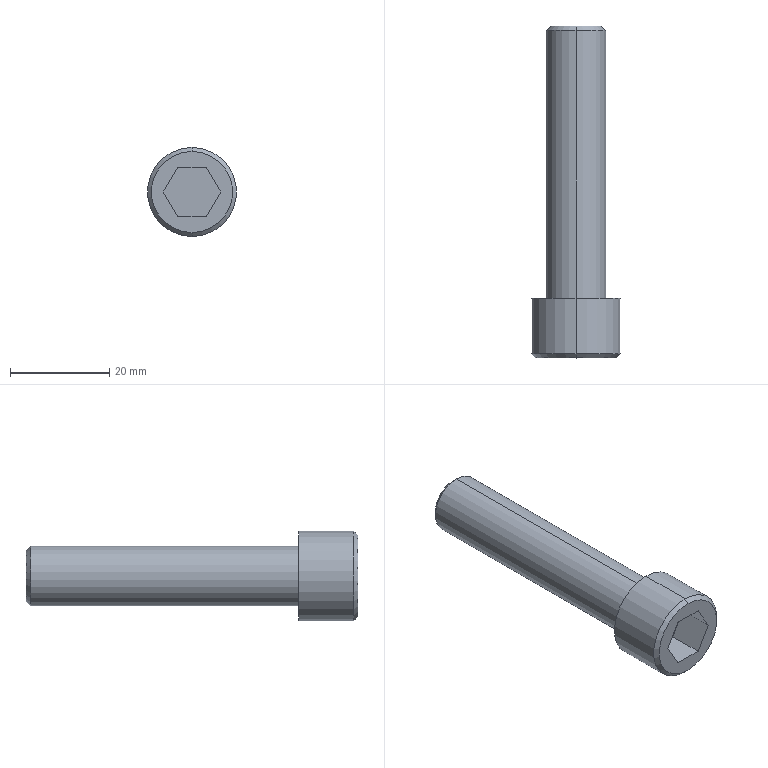Part | Creo | 1 solid | 18 faces | box 18 x 67 x 18 mm | volume 8618 mm3 | plane 10 | cylinder 4 | cone 4 | commonest cylinder face diameters 12 x2 18 x2
STEP:
#1=CARTESIAN_POINT('',(244.,-386.,-274.));
#2=VERTEX_POINT('',#1);
#3=CARTESIAN_POINT('',(244.,-386.,-292.));
#4=VERTEX_POINT('',#3);
#5=CARTESIAN_POINT('',(244.,-386.,-283.));
#6=DIRECTION('',(0.,1.,0.));
#7=DIRECTION('',(0.,0.,1.));
#8=AXIS2_PLACEMENT_3D('',#5,#6,#7);
#9=CIRCLE('',#8,9.);
#10=EDGE_CURVE('',#2,#4,#9,.T.);
#11=ORIENTED_EDGE('',*,*,#10,.F.);
#12=CARTESIAN_POINT('',(244.,-386.,-283.));
#13=DIRECTION('',(0.,1.,0.));
#14=DIRECTION('',(0.,0.,-1.));
#15=AXIS2_PLACEMENT_3D('',#12,#13,#14);
#16=CIRCLE('',#15,9.);
#17=EDGE_CURVE('',#4,#2,#16,.T.);
#18=ORIENTED_EDGE('',*,*,#17,.F.);
#19=EDGE_LOOP('',(#11,#18));
#20=FACE_OUTER_BOUND('',#19,.F.);
#21=CARTESIAN_POINT('',(244.,-386.,-277.));
#22=VERTEX_POINT('',#21);
#23=CARTESIAN_POINT('',(244.,-386.,-289.));
#24=VERTEX_POINT('',#23);
#25=CARTESIAN_POINT('',(244.,-386.,-283.));
#26=DIRECTION('',(0.,-1.,0.));
#27=DIRECTION('',(0.,0.,1.));
#28=AXIS2_PLACEMENT_3D('',#25,#26,#27);
#29=CIRCLE('',#28,6.);
#30=EDGE_CURVE('',#22,#24,#29,.T.);
#31=ORIENTED_EDGE('',*,*,#30,.F.);
#32=CARTESIAN_POINT('',(244.,-386.,-283.));
#33=DIRECTION('',(0.,-1.,0.));
#34=DIRECTION('',(0.,0.,-1.));
#35=AXIS2_PLACEMENT_3D('',#32,#33,#34);
#36=CIRCLE('',#35,6.);
#37=EDGE_CURVE('',#24,#22,#36,.T.);
#38=ORIENTED_EDGE('',*,*,#37,.F.);
#39=EDGE_LOOP('',(#31,#38));
#40=FACE_BOUND('',#39,.F.);
#41=CARTESIAN_POINT('',(244.,-386.,-283.));
#42=DIRECTION('',(0.,1.,0.));
#43=DIRECTION('',(0.,0.,-1.));
#44=AXIS2_PLACEMENT_3D('',#41,#42,#43);
#45=PLANE('',#44);
#46=ADVANCED_FACE('',(#20,#40),#45,.T.);
#47=CARTESIAN_POINT('',(244.,-331.9,-289.));
#48=VERTEX_POINT('',#47);
#49=CARTESIAN_POINT('',(244.,-331.9,-277.));
#50=VERTEX_POINT('',#49);
#51=CARTESIAN_POINT('',(244.,-331.9,-283.));
#52=DIRECTION('',(0.,1.,0.));
#53=DIRECTION('',(0.,0.,-1.));
#54=AXIS2_PLACEMENT_3D('',#51,#52,#53);
#55=CIRCLE('',#54,6.);
#56=EDGE_CURVE('',#48,#50,#55,.T.);
#57=ORIENTED_EDGE('',*,*,#56,.T.);
#58=CARTESIAN_POINT('',(244.,-386.,-277.));
#59=DIRECTION('',(0.,1.,0.));
#60=VECTOR('',#59,54.1);
#61=LINE('',#58,#60);
#62=EDGE_CURVE('',#22,#50,#61,.T.);
#63=ORIENTED_EDGE('',*,*,#62,.F.);
#64=ORIENTED_EDGE('',*,*,#30,.T.);
#65=CARTESIAN_POINT('',(244.,-386.,-289.));
#66=DIRECTION('',(0.,1.,0.));
#67=VECTOR('',#66,54.1);
#68=LINE('',#65,#67);
#69=EDGE_CURVE('',#24,#48,#68,.T.);
#70=ORIENTED_EDGE('',*,*,#69,.T.);
#71=EDGE_LOOP('',(#57,#63,#64,#70));
#72=FACE_OUTER_BOUND('',#71,.F.);
#73=CARTESIAN_POINT('',(244.,-400.,-283.));
#74=DIRECTION('',(0.,1.,0.));
#75=DIRECTION('',(0.,0.,-1.));
#76=AXIS2_PLACEMENT_3D('',#73,#74,#75);
#77=CYLINDRICAL_SURFACE('',#76,6.);
#78=ADVANCED_FACE('',(#72),#77,.T.);
#79=CARTESIAN_POINT('',(244.,-331.,-288.1));
#80=VERTEX_POINT('',#79);
#81=CARTESIAN_POINT('',(244.,-331.,-277.9));
#82=VERTEX_POINT('',#81);
#83=CARTESIAN_POINT('',(244.,-331.,-283.));
#84=DIRECTION('',(0.,1.,0.));
#85=DIRECTION('',(0.,0.,-1.));
#86=AXIS2_PLACEMENT_3D('',#83,#84,#85);
#87=CIRCLE('',#86,5.1);
#88=EDGE_CURVE('',#80,#82,#87,.T.);
#89=ORIENTED_EDGE('',*,*,#88,.T.);
#90=CARTESIAN_POINT('',(244.,-331.,-277.9));
#91=DIRECTION('',(0.,-0.7071,0.7071));
#92=VECTOR('',#91,1.273);
#93=LINE('',#90,#92);
#94=EDGE_CURVE('',#82,#50,#93,.T.);
#95=ORIENTED_EDGE('',*,*,#94,.T.);
#96=ORIENTED_EDGE('',*,*,#56,.F.);
#97=CARTESIAN_POINT('',(244.,-331.,-288.1));
#98=DIRECTION('',(0.,-0.7071,-0.7071));
#99=VECTOR('',#98,1.273);
#100=LINE('',#97,#99);
#101=EDGE_CURVE('',#80,#48,#100,.T.);
#102=ORIENTED_EDGE('',*,*,#101,.F.);
#103=EDGE_LOOP('',(#89,#95,#96,#102));
#104=FACE_OUTER_BOUND('',#103,.F.);
#105=CARTESIAN_POINT('',(244.,-331.45,-283.));
#106=DIRECTION('',(0.,-1.,0.));
#107=DIRECTION('',(0.,0.,-1.));
#108=AXIS2_PLACEMENT_3D('',#105,#106,#107);
#109=CONICAL_SURFACE('',#108,5.55,45.);
#110=ADVANCED_FACE('',(#104),#109,.T.);
#111=CARTESIAN_POINT('',(244.,-331.,-283.));
#112=DIRECTION('',(0.,1.,0.));
#113=DIRECTION('',(0.,0.,1.));
#114=AXIS2_PLACEMENT_3D('',#111,#112,#113);
#115=CIRCLE('',#114,5.1);
#116=EDGE_CURVE('',#82,#80,#115,.T.);
#117=ORIENTED_EDGE('',*,*,#116,.F.);
#118=ORIENTED_EDGE('',*,*,#88,.F.);
#119=EDGE_LOOP('',(#117,#118));
#120=FACE_OUTER_BOUND('',#119,.F.);
#121=CARTESIAN_POINT('',(244.,-331.,-283.));
#122=DIRECTION('',(0.,1.,0.));
#123=DIRECTION('',(0.,0.,-1.));
#124=AXIS2_PLACEMENT_3D('',#121,#122,#123);
#125=PLANE('',#124);
#126=ADVANCED_FACE('',(#120),#125,.T.);
#127=ORIENTED_EDGE('',*,*,#116,.T.);
#128=ORIENTED_EDGE('',*,*,#101,.T.);
#129=CARTESIAN_POINT('',(244.,-331.9,-283.));
#130=DIRECTION('',(0.,1.,0.));
#131=DIRECTION('',(0.,0.,1.));
#132=AXIS2_PLACEMENT_3D('',#129,#130,#131);
#133=CIRCLE('',#132,6.);
#134=EDGE_CURVE('',#50,#48,#133,.T.);
#135=ORIENTED_EDGE('',*,*,#134,.F.);
#136=ORIENTED_EDGE('',*,*,#94,.F.);
#137=EDGE_LOOP('',(#127,#128,#135,#136));
#138=FACE_OUTER_BOUND('',#137,.F.);
#139=CARTESIAN_POINT('',(244.,-331.45,-283.));
#140=DIRECTION('',(0.,-1.,0.));
#141=DIRECTION('',(0.,0.,-1.));
#142=AXIS2_PLACEMENT_3D('',#139,#140,#141);
#143=CONICAL_SURFACE('',#142,5.55,45.);
#144=ADVANCED_FACE('',(#138),#143,.T.);
#145=ORIENTED_EDGE('',*,*,#134,.T.);
#146=ORIENTED_EDGE('',*,*,#69,.F.);
#147=ORIENTED_EDGE('',*,*,#37,.T.);
#148=ORIENTED_EDGE('',*,*,#62,.T.);
#149=EDGE_LOOP('',(#145,#146,#147,#148));
#150=FACE_OUTER_BOUND('',#149,.F.);
#151=CARTESIAN_POINT('',(244.,-400.,-283.));
#152=DIRECTION('',(0.,1.,0.));
#153=DIRECTION('',(0.,0.,-1.));
#154=AXIS2_PLACEMENT_3D('',#151,#152,#153);
#155=CYLINDRICAL_SURFACE('',#154,6.);
#156=ADVANCED_FACE('',(#150),#155,.T.);
#157=CARTESIAN_POINT('',(244.,-397.2,-292.));
#158=VERTEX_POINT('',#157);
#159=CARTESIAN_POINT('',(244.,-397.2,-274.));
#160=VERTEX_POINT('',#159);
#161=CARTESIAN_POINT('',(244.,-397.2,-283.));
#162=DIRECTION('',(0.,-1.,0.));
#163=DIRECTION('',(0.,0.,-1.));
#164=AXIS2_PLACEMENT_3D('',#161,#162,#163);
#165=CIRCLE('',#164,9.);
#166=EDGE_CURVE('',#158,#160,#165,.T.);
#167=ORIENTED_EDGE('',*,*,#166,.T.);
#168=CARTESIAN_POINT('',(244.,-397.2,-274.));
#169=DIRECTION('',(0.,1.,0.));
#170=VECTOR('',#169,11.2);
#171=LINE('',#168,#170);
#172=EDGE_CURVE('',#160,#2,#171,.T.);
#173=ORIENTED_EDGE('',*,*,#172,.T.);
#174=ORIENTED_EDGE('',*,*,#10,.T.);
#175=CARTESIAN_POINT('',(244.,-397.2,-292.));
#176=DIRECTION('',(0.,1.,0.));
#177=VECTOR('',#176,11.2);
#178=LINE('',#175,#177);
#179=EDGE_CURVE('',#158,#4,#178,.T.);
#180=ORIENTED_EDGE('',*,*,#179,.F.);
#181=EDGE_LOOP('',(#167,#173,#174,#180));
#182=FACE_OUTER_BOUND('',#181,.F.);
#183=CARTESIAN_POINT('',(244.,-400.,-283.));
#184=DIRECTION('',(0.,1.,0.));
#185=DIRECTION('',(0.,0.,-1.));
#186=AXIS2_PLACEMENT_3D('',#183,#184,#185);
#187=CYLINDRICAL_SURFACE('',#186,9.);
#188=ADVANCED_FACE('',(#182),#187,.T.);
#189=CARTESIAN_POINT('',(244.,-398.,-291.2));
#190=VERTEX_POINT('',#189);
#191=CARTESIAN_POINT('',(244.,-398.,-274.8));
#192=VERTEX_POINT('',#191);
#193=CARTESIAN_POINT('',(244.,-398.,-283.));
#194=DIRECTION('',(0.,-1.,0.));
#195=DIRECTION('',(0.,0.,-1.));
#196=AXIS2_PLACEMENT_3D('',#193,#194,#195);
#197=CIRCLE('',#196,8.2);
#198=EDGE_CURVE('',#190,#192,#197,.T.);
#199=ORIENTED_EDGE('',*,*,#198,.T.);
#200=CARTESIAN_POINT('',(244.,-398.,-274.8));
#201=DIRECTION('',(0.,0.7071,0.7071));
#202=VECTOR('',#201,1.131);
#203=LINE('',#200,#202);
#204=EDGE_CURVE('',#192,#160,#203,.T.);
#205=ORIENTED_EDGE('',*,*,#204,.T.);
#206=ORIENTED_EDGE('',*,*,#166,.F.);
#207=CARTESIAN_POINT('',(244.,-398.,-291.2));
#208=DIRECTION('',(0.,0.7071,-0.7071));
#209=VECTOR('',#208,1.131);
#210=LINE('',#207,#209);
#211=EDGE_CURVE('',#190,#158,#210,.T.);
#212=ORIENTED_EDGE('',*,*,#211,.F.);
#213=EDGE_LOOP('',(#199,#205,#206,#212));
#214=FACE_OUTER_BOUND('',#213,.F.);
#215=CARTESIAN_POINT('',(244.,-397.6,-283.));
#216=DIRECTION('',(0.,1.,0.));
#217=DIRECTION('',(0.,0.,1.));
#218=AXIS2_PLACEMENT_3D('',#215,#216,#217);
#219=CONICAL_SURFACE('',#218,8.6,45.);
#220=ADVANCED_FACE('',(#214),#219,.T.);
#221=CARTESIAN_POINT('',(244.,-398.,-283.));
#222=DIRECTION('',(0.,-1.,0.));
#223=DIRECTION('',(0.,0.,1.));
#224=AXIS2_PLACEMENT_3D('',#221,#222,#223);
#225=CIRCLE('',#224,8.2);
#226=EDGE_CURVE('',#192,#190,#225,.T.);
#227=ORIENTED_EDGE('',*,*,#226,.F.);
#228=ORIENTED_EDGE('',*,*,#198,.F.);
#229=EDGE_LOOP('',(#227,#228));
#230=FACE_OUTER_BOUND('',#229,.F.);
#231=CARTESIAN_POINT('',(246.887,-398.,-278.));
#232=VERTEX_POINT('',#231);
#233=CARTESIAN_POINT('',(249.774,-398.,-283.));
#234=VERTEX_POINT('',#233);
#235=CARTESIAN_POINT('',(246.887,-398.,-278.));
#236=DIRECTION('',(0.5,0.,-0.866));
#237=VECTOR('',#236,5.774);
#238=LINE('',#235,#237);
#239=EDGE_CURVE('',#232,#234,#238,.T.);
#240=ORIENTED_EDGE('',*,*,#239,.F.);
#241=CARTESIAN_POINT('',(241.113,-398.,-278.));
#242=VERTEX_POINT('',#241);
#243=CARTESIAN_POINT('',(241.113,-398.,-278.));
#244=DIRECTION('',(1.,0.,0.));
#245=VECTOR('',#244,5.774);
#246=LINE('',#243,#245);
#247=EDGE_CURVE('',#242,#232,#246,.T.);
#248=ORIENTED_EDGE('',*,*,#247,.F.);
#249=CARTESIAN_POINT('',(238.226,-398.,-283.));
#250=VERTEX_POINT('',#249);
#251=CARTESIAN_POINT('',(238.226,-398.,-283.));
#252=DIRECTION('',(0.5,0.,0.866));
#253=VECTOR('',#252,5.774);
#254=LINE('',#251,#253);
#255=EDGE_CURVE('',#250,#242,#254,.T.);
#256=ORIENTED_EDGE('',*,*,#255,.F.);
#257=CARTESIAN_POINT('',(241.113,-398.,-288.));
#258=VERTEX_POINT('',#257);
#259=CARTESIAN_POINT('',(241.113,-398.,-288.));
#260=DIRECTION('',(-0.5,0.,0.866));
#261=VECTOR('',#260,5.774);
#262=LINE('',#259,#261);
#263=EDGE_CURVE('',#258,#250,#262,.T.);
#264=ORIENTED_EDGE('',*,*,#263,.F.);
#265=CARTESIAN_POINT('',(246.887,-398.,-288.));
#266=VERTEX_POINT('',#265);
#267=CARTESIAN_POINT('',(246.887,-398.,-288.));
#268=DIRECTION('',(-1.,0.,0.));
#269=VECTOR('',#268,5.774);
#270=LINE('',#267,#269);
#271=EDGE_CURVE('',#266,#258,#270,.T.);
#272=ORIENTED_EDGE('',*,*,#271,.F.);
#273=CARTESIAN_POINT('',(249.774,-398.,-283.));
#274=DIRECTION('',(-0.5,0.,-0.866));
#275=VECTOR('',#274,5.774);
#276=LINE('',#273,#275);
#277=EDGE_CURVE('',#234,#266,#276,.T.);
#278=ORIENTED_EDGE('',*,*,#277,.F.);
#279=EDGE_LOOP('',(#240,#248,#256,#264,#272,#278));
#280=FACE_BOUND('',#279,.F.);
#281=CARTESIAN_POINT('',(244.,-398.,-283.));
#282=DIRECTION('',(0.,1.,0.));
#283=DIRECTION('',(0.,0.,1.));
#284=AXIS2_PLACEMENT_3D('',#281,#282,#283);
#285=PLANE('',#284);
#286=ADVANCED_FACE('',(#230,#280),#285,.F.);
#287=ORIENTED_EDGE('',*,*,#226,.T.);
#288=ORIENTED_EDGE('',*,*,#211,.T.);
#289=CARTESIAN_POINT('',(244.,-397.2,-283.));
#290=DIRECTION('',(0.,-1.,0.));
#291=DIRECTION('',(0.,0.,1.));
#292=AXIS2_PLACEMENT_3D('',#289,#290,#291);
#293=CIRCLE('',#292,9.);
#294=EDGE_CURVE('',#160,#158,#293,.T.);
#295=ORIENTED_EDGE('',*,*,#294,.F.);
#296=ORIENTED_EDGE('',*,*,#204,.F.);
#297=EDGE_LOOP('',(#287,#288,#295,#296));
#298=FACE_OUTER_BOUND('',#297,.F.);
#299=CARTESIAN_POINT('',(244.,-397.6,-283.));
#300=DIRECTION('',(0.,1.,0.));
#301=DIRECTION('',(0.,0.,1.));
#302=AXIS2_PLACEMENT_3D('',#299,#300,#301);
#303=CONICAL_SURFACE('',#302,8.6,45.);
#304=ADVANCED_FACE('',(#298),#303,.T.);
#305=ORIENTED_EDGE('',*,*,#294,.T.);
#306=ORIENTED_EDGE('',*,*,#179,.T.);
#307=ORIENTED_EDGE('',*,*,#17,.T.);
#308=ORIENTED_EDGE('',*,*,#172,.F.);
#309=EDGE_LOOP('',(#305,#306,#307,#308));
#310=FACE_OUTER_BOUND('',#309,.F.);
#311=CARTESIAN_POINT('',(244.,-400.,-283.));
#312=DIRECTION('',(0.,1.,0.));
#313=DIRECTION('',(0.,0.,-1.));
#314=AXIS2_PLACEMENT_3D('',#311,#312,#313);
#315=CYLINDRICAL_SURFACE('',#314,9.);
#316=ADVANCED_FACE('',(#310),#315,.T.);
#317=ORIENTED_EDGE('',*,*,#239,.T.);
#318=CARTESIAN_POINT('',(249.774,-390.8,-283.));
#319=VERTEX_POINT('',#318);
#320=CARTESIAN_POINT('',(249.774,-398.,-283.));
#321=DIRECTION('',(0.,1.,0.));
#322=VECTOR('',#321,7.2);
#323=LINE('',#320,#322);
#324=EDGE_CURVE('',#234,#319,#323,.T.);
#325=ORIENTED_EDGE('',*,*,#324,.T.);
#326=CARTESIAN_POINT('',(246.887,-390.8,-278.));
#327=VERTEX_POINT('',#326);
#328=CARTESIAN_POINT('',(249.774,-390.8,-283.));
#329=DIRECTION('',(-0.5,0.,0.866));
#330=VECTOR('',#329,5.774);
#331=LINE('',#328,#330);
#332=EDGE_CURVE('',#319,#327,#331,.T.);
#333=ORIENTED_EDGE('',*,*,#332,.T.);
#334=CARTESIAN_POINT('',(246.887,-398.,-278.));
#335=DIRECTION('',(0.,1.,0.));
#336=VECTOR('',#335,7.2);
#337=LINE('',#334,#336);
#338=EDGE_CURVE('',#232,#327,#337,.T.);
#339=ORIENTED_EDGE('',*,*,#338,.F.);
#340=EDGE_LOOP('',(#317,#325,#333,#339));
#341=FACE_OUTER_BOUND('',#340,.F.);
#342=CARTESIAN_POINT('',(249.774,-390.8,-283.));
#343=DIRECTION('',(0.866,0.,0.5));
#344=DIRECTION('',(0.5,0.,-0.866));
#345=AXIS2_PLACEMENT_3D('',#342,#343,#344);
#346=PLANE('',#345);
#347=ADVANCED_FACE('',(#341),#346,.F.);
#348=ORIENTED_EDGE('',*,*,#277,.T.);
#349=CARTESIAN_POINT('',(246.887,-390.8,-288.));
#350=VERTEX_POINT('',#349);
#351=CARTESIAN_POINT('',(246.887,-398.,-288.));
#352=DIRECTION('',(0.,1.,0.));
#353=VECTOR('',#352,7.2);
#354=LINE('',#351,#353);
#355=EDGE_CURVE('',#266,#350,#354,.T.);
#356=ORIENTED_EDGE('',*,*,#355,.T.);
#357=CARTESIAN_POINT('',(246.887,-390.8,-288.));
#358=DIRECTION('',(0.5,0.,0.866));
#359=VECTOR('',#358,5.774);
#360=LINE('',#357,#359);
#361=EDGE_CURVE('',#350,#319,#360,.T.);
#362=ORIENTED_EDGE('',*,*,#361,.T.);
#363=ORIENTED_EDGE('',*,*,#324,.F.);
#364=EDGE_LOOP('',(#348,#356,#362,#363));
#365=FACE_OUTER_BOUND('',#364,.F.);
#366=CARTESIAN_POINT('',(246.887,-390.8,-288.));
#367=DIRECTION('',(0.866,0.,-0.5));
#368=DIRECTION('',(-0.5,0.,-0.866));
#369=AXIS2_PLACEMENT_3D('',#366,#367,#368);
#370=PLANE('',#369);
#371=ADVANCED_FACE('',(#365),#370,.F.);
#372=ORIENTED_EDGE('',*,*,#271,.T.);
#373=CARTESIAN_POINT('',(241.113,-390.8,-288.));
#374=VERTEX_POINT('',#373);
#375=CARTESIAN_POINT('',(241.113,-398.,-288.));
#376=DIRECTION('',(0.,1.,0.));
#377=VECTOR('',#376,7.2);
#378=LINE('',#375,#377);
#379=EDGE_CURVE('',#258,#374,#378,.T.);
#380=ORIENTED_EDGE('',*,*,#379,.T.);
#381=CARTESIAN_POINT('',(246.887,-390.8,-288.));
#382=DIRECTION('',(-1.,0.,0.));
#383=VECTOR('',#382,5.774);
#384=LINE('',#381,#383);
#385=EDGE_CURVE('',#350,#374,#384,.T.);
#386=ORIENTED_EDGE('',*,*,#385,.F.);
#387=ORIENTED_EDGE('',*,*,#355,.F.);
#388=EDGE_LOOP('',(#372,#380,#386,#387));
#389=FACE_OUTER_BOUND('',#388,.F.);
#390=CARTESIAN_POINT('',(241.113,-390.8,-288.));
#391=DIRECTION('',(0.,0.,-1.));
#392=DIRECTION('',(-1.,0.,0.));
#393=AXIS2_PLACEMENT_3D('',#390,#391,#392);
#394=PLANE('',#393);
#395=ADVANCED_FACE('',(#389),#394,.F.);
#396=ORIENTED_EDGE('',*,*,#263,.T.);
#397=CARTESIAN_POINT('',(238.226,-390.8,-283.));
#398=VERTEX_POINT('',#397);
#399=CARTESIAN_POINT('',(238.226,-398.,-283.));
#400=DIRECTION('',(0.,1.,0.));
#401=VECTOR('',#400,7.2);
#402=LINE('',#399,#401);
#403=EDGE_CURVE('',#250,#398,#402,.T.);
#404=ORIENTED_EDGE('',*,*,#403,.T.);
#405=CARTESIAN_POINT('',(238.226,-390.8,-283.));
#406=DIRECTION('',(0.5,0.,-0.866));
#407=VECTOR('',#406,5.774);
#408=LINE('',#405,#407);
#409=EDGE_CURVE('',#398,#374,#408,.T.);
#410=ORIENTED_EDGE('',*,*,#409,.T.);
#411=ORIENTED_EDGE('',*,*,#379,.F.);
#412=EDGE_LOOP('',(#396,#404,#410,#411));
#413=FACE_OUTER_BOUND('',#412,.F.);
#414=CARTESIAN_POINT('',(238.226,-390.8,-283.));
#415=DIRECTION('',(-0.866,0.,-0.5));
#416=DIRECTION('',(-0.5,0.,0.866));
#417=AXIS2_PLACEMENT_3D('',#414,#415,#416);
#418=PLANE('',#417);
#419=ADVANCED_FACE('',(#413),#418,.F.);
#420=ORIENTED_EDGE('',*,*,#255,.T.);
#421=CARTESIAN_POINT('',(241.113,-390.8,-278.));
#422=VERTEX_POINT('',#421);
#423=CARTESIAN_POINT('',(241.113,-398.,-278.));
#424=DIRECTION('',(0.,1.,0.));
#425=VECTOR('',#424,7.2);
#426=LINE('',#423,#425);
#427=EDGE_CURVE('',#242,#422,#426,.T.);
#428=ORIENTED_EDGE('',*,*,#427,.T.);
#429=CARTESIAN_POINT('',(241.113,-390.8,-278.));
#430=DIRECTION('',(-0.5,0.,-0.866));
#431=VECTOR('',#430,5.774);
#432=LINE('',#429,#431);
#433=EDGE_CURVE('',#422,#398,#432,.T.);
#434=ORIENTED_EDGE('',*,*,#433,.T.);
#435=ORIENTED_EDGE('',*,*,#403,.F.);
#436=EDGE_LOOP('',(#420,#428,#434,#435));
#437=FACE_OUTER_BOUND('',#436,.F.);
#438=CARTESIAN_POINT('',(241.113,-390.8,-278.));
#439=DIRECTION('',(-0.866,0.,0.5));
#440=DIRECTION('',(0.5,0.,0.866));
#441=AXIS2_PLACEMENT_3D('',#438,#439,#440);
#442=PLANE('',#441);
#443=ADVANCED_FACE('',(#437),#442,.F.);
#444=ORIENTED_EDGE('',*,*,#247,.T.);
#445=ORIENTED_EDGE('',*,*,#338,.T.);
#446=CARTESIAN_POINT('',(241.113,-390.8,-278.));
#447=DIRECTION('',(1.,0.,0.));
#448=VECTOR('',#447,5.774);
#449=LINE('',#446,#448);
#450=EDGE_CURVE('',#422,#327,#449,.T.);
#451=ORIENTED_EDGE('',*,*,#450,.F.);
#452=ORIENTED_EDGE('',*,*,#427,.F.);
#453=EDGE_LOOP('',(#444,#445,#451,#452));
#454=FACE_OUTER_BOUND('',#453,.F.);
#455=CARTESIAN_POINT('',(246.887,-390.8,-278.));
#456=DIRECTION('',(0.,0.,1.));
#457=DIRECTION('',(1.,0.,0.));
#458=AXIS2_PLACEMENT_3D('',#455,#456,#457);
#459=PLANE('',#458);
#460=ADVANCED_FACE('',(#454),#459,.F.);
#461=ORIENTED_EDGE('',*,*,#361,.F.);
#462=ORIENTED_EDGE('',*,*,#385,.T.);
#463=ORIENTED_EDGE('',*,*,#409,.F.);
#464=ORIENTED_EDGE('',*,*,#433,.F.);
#465=ORIENTED_EDGE('',*,*,#450,.T.);
#466=ORIENTED_EDGE('',*,*,#332,.F.);
#467=EDGE_LOOP('',(#461,#462,#463,#464,#465,#466));
#468=FACE_OUTER_BOUND('',#467,.F.);
#469=CARTESIAN_POINT('',(249.774,-390.8,-283.));
#470=DIRECTION('',(0.,-1.,0.));
#471=DIRECTION('',(0.,0.,-1.));
#472=AXIS2_PLACEMENT_3D('',#469,#470,#471);
#473=PLANE('',#472);
#474=ADVANCED_FACE('',(#468),#473,.T.);
#475=CLOSED_SHELL('',(#46,#78,#110,#126,#144,#156,#188,#220,#286,#304,#316,#347,#371,#395,#419,#443,#460,#474));
#476=MANIFOLD_SOLID_BREP('',#475);
#477=(LENGTH_UNIT()NAMED_UNIT(*)SI_UNIT(.MILLI.,.METRE.));
#478=UNCERTAINTY_MEASURE_WITH_UNIT(LENGTH_MEASURE(0.007167),#477,'','');
#479=(NAMED_UNIT(*)PLANE_ANGLE_UNIT()SI_UNIT($,.RADIAN.));
#480=PLANE_ANGLE_MEASURE_WITH_UNIT(PLANE_ANGLE_MEASURE(0.01745),#479);
#481=(CONVERSION_BASED_UNIT('DEGREE',#480)NAMED_UNIT(*)PLANE_ANGLE_UNIT());
#482=(NAMED_UNIT(*)SI_UNIT($,.STERADIAN.)SOLID_ANGLE_UNIT());
#483=(GEOMETRIC_REPRESENTATION_CONTEXT(3)GLOBAL_UNCERTAINTY_ASSIGNED_CONTEXT((#478))GLOBAL_UNIT_ASSIGNED_CONTEXT((#477,#481,#482))REPRESENTATION_CONTEXT('',''));
#484=ADVANCED_BREP_SHAPE_REPRESENTATION('',(#476),#483);